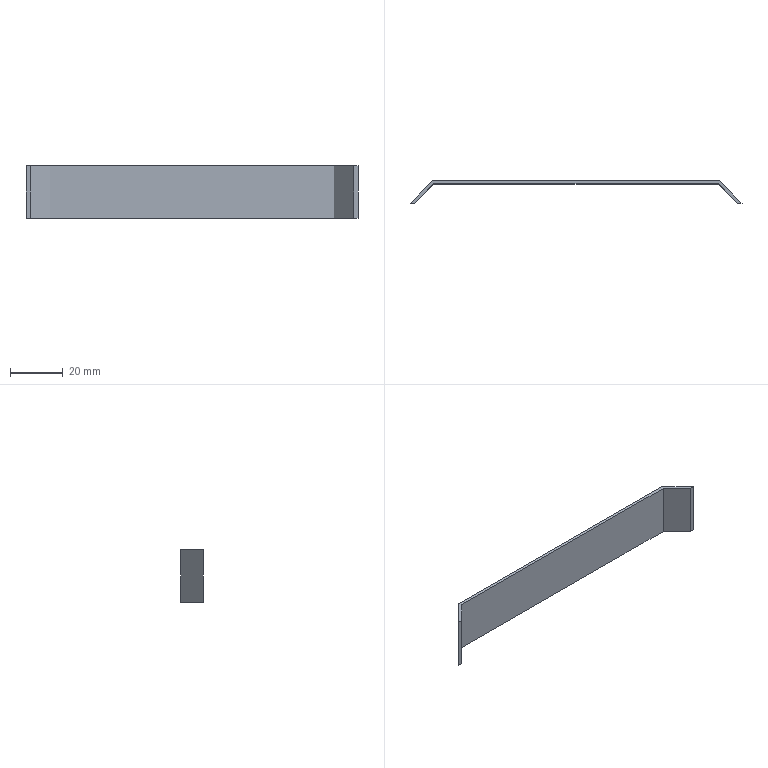Part | SolidWorks | features BaseBody 1 | 1 solid | 10 faces | box 126 x 8.5 x 20 mm | volume 3140 mm3 | plane 10
STEP:
#1=CARTESIAN_POINT('',(63.,-8.5,-10.));
#2=VERTEX_POINT('',#1);
#3=CARTESIAN_POINT('',(54.5,0.,-10.));
#4=VERTEX_POINT('',#3);
#5=CARTESIAN_POINT('',(54.5,0.,-10.));
#6=DIRECTION('',(-0.7071,0.7071,0.));
#7=VECTOR('',#6,1000.);
#8=LINE('',#5,#7);
#9=EDGE_CURVE('',#2,#4,#8,.T.);
#10=ORIENTED_EDGE('',*,*,#9,.F.);
#11=CARTESIAN_POINT('',(61.303,-8.5,-10.));
#12=VERTEX_POINT('',#11);
#13=CARTESIAN_POINT('',(63.,-8.5,-10.));
#14=DIRECTION('',(1.,0.,0.));
#15=VECTOR('',#14,1000.);
#16=LINE('',#13,#15);
#17=EDGE_CURVE('',#12,#2,#16,.T.);
#18=ORIENTED_EDGE('',*,*,#17,.F.);
#19=CARTESIAN_POINT('',(54.003,-1.2,-10.));
#20=VERTEX_POINT('',#19);
#21=CARTESIAN_POINT('',(54.003,-1.2,-10.));
#22=DIRECTION('',(0.7071,-0.7071,0.));
#23=VECTOR('',#22,1000.);
#24=LINE('',#21,#23);
#25=EDGE_CURVE('',#20,#12,#24,.T.);
#26=ORIENTED_EDGE('',*,*,#25,.F.);
#27=CARTESIAN_POINT('',(-54.003,-1.2,-10.));
#28=VERTEX_POINT('',#27);
#29=CARTESIAN_POINT('',(0.,-1.2,-10.));
#30=DIRECTION('',(1.,0.,0.));
#31=VECTOR('',#30,1000.);
#32=LINE('',#29,#31);
#33=EDGE_CURVE('',#28,#20,#32,.T.);
#34=ORIENTED_EDGE('',*,*,#33,.F.);
#35=CARTESIAN_POINT('',(-61.303,-8.5,-10.));
#36=VERTEX_POINT('',#35);
#37=CARTESIAN_POINT('',(-54.003,-1.2,-10.));
#38=DIRECTION('',(0.7071,0.7071,0.));
#39=VECTOR('',#38,1000.);
#40=LINE('',#37,#39);
#41=EDGE_CURVE('',#36,#28,#40,.T.);
#42=ORIENTED_EDGE('',*,*,#41,.F.);
#43=CARTESIAN_POINT('',(-63.,-8.5,-10.));
#44=VERTEX_POINT('',#43);
#45=CARTESIAN_POINT('',(-63.,-8.5,-10.));
#46=DIRECTION('',(1.,0.,0.));
#47=VECTOR('',#46,1000.);
#48=LINE('',#45,#47);
#49=EDGE_CURVE('',#44,#36,#48,.T.);
#50=ORIENTED_EDGE('',*,*,#49,.F.);
#51=CARTESIAN_POINT('',(-54.5,0.,-10.));
#52=VERTEX_POINT('',#51);
#53=CARTESIAN_POINT('',(-54.5,0.,-10.));
#54=DIRECTION('',(-0.7071,-0.7071,0.));
#55=VECTOR('',#54,1000.);
#56=LINE('',#53,#55);
#57=EDGE_CURVE('',#52,#44,#56,.T.);
#58=ORIENTED_EDGE('',*,*,#57,.F.);
#59=CARTESIAN_POINT('',(0.,0.,-10.));
#60=DIRECTION('',(-1.,0.,0.));
#61=VECTOR('',#60,1000.);
#62=LINE('',#59,#61);
#63=EDGE_CURVE('',#4,#52,#62,.T.);
#64=ORIENTED_EDGE('',*,*,#63,.F.);
#65=EDGE_LOOP('',(#10,#18,#26,#34,#42,#50,#58,#64));
#66=FACE_OUTER_BOUND('',#65,.T.);
#67=CARTESIAN_POINT('',(0.,0.,-10.));
#68=DIRECTION('',(0.,0.,-1.));
#69=DIRECTION('',(0.,-1.,0.));
#70=AXIS2_PLACEMENT_3D('',#67,#68,#69);
#71=PLANE('',#70);
#72=ADVANCED_FACE('',(#66),#71,.T.);
#73=CARTESIAN_POINT('',(63.,-8.5,10.));
#74=VERTEX_POINT('',#73);
#75=CARTESIAN_POINT('',(54.5,0.,10.));
#76=VERTEX_POINT('',#75);
#77=CARTESIAN_POINT('',(54.5,0.,10.));
#78=DIRECTION('',(-0.7071,0.7071,0.));
#79=VECTOR('',#78,1000.);
#80=LINE('',#77,#79);
#81=EDGE_CURVE('',#74,#76,#80,.T.);
#82=ORIENTED_EDGE('',*,*,#81,.T.);
#83=CARTESIAN_POINT('',(-54.5,0.,10.));
#84=VERTEX_POINT('',#83);
#85=CARTESIAN_POINT('',(0.,0.,10.));
#86=DIRECTION('',(-1.,0.,0.));
#87=VECTOR('',#86,1000.);
#88=LINE('',#85,#87);
#89=EDGE_CURVE('',#76,#84,#88,.T.);
#90=ORIENTED_EDGE('',*,*,#89,.T.);
#91=CARTESIAN_POINT('',(-63.,-8.5,10.));
#92=VERTEX_POINT('',#91);
#93=CARTESIAN_POINT('',(-54.5,0.,10.));
#94=DIRECTION('',(-0.7071,-0.7071,0.));
#95=VECTOR('',#94,1000.);
#96=LINE('',#93,#95);
#97=EDGE_CURVE('',#84,#92,#96,.T.);
#98=ORIENTED_EDGE('',*,*,#97,.T.);
#99=CARTESIAN_POINT('',(-61.303,-8.5,10.));
#100=VERTEX_POINT('',#99);
#101=CARTESIAN_POINT('',(-63.,-8.5,10.));
#102=DIRECTION('',(1.,0.,0.));
#103=VECTOR('',#102,1000.);
#104=LINE('',#101,#103);
#105=EDGE_CURVE('',#92,#100,#104,.T.);
#106=ORIENTED_EDGE('',*,*,#105,.T.);
#107=CARTESIAN_POINT('',(-54.003,-1.2,10.));
#108=VERTEX_POINT('',#107);
#109=CARTESIAN_POINT('',(-54.003,-1.2,10.));
#110=DIRECTION('',(0.7071,0.7071,0.));
#111=VECTOR('',#110,1000.);
#112=LINE('',#109,#111);
#113=EDGE_CURVE('',#100,#108,#112,.T.);
#114=ORIENTED_EDGE('',*,*,#113,.T.);
#115=CARTESIAN_POINT('',(54.003,-1.2,10.));
#116=VERTEX_POINT('',#115);
#117=CARTESIAN_POINT('',(0.,-1.2,10.));
#118=DIRECTION('',(1.,0.,0.));
#119=VECTOR('',#118,1000.);
#120=LINE('',#117,#119);
#121=EDGE_CURVE('',#108,#116,#120,.T.);
#122=ORIENTED_EDGE('',*,*,#121,.T.);
#123=CARTESIAN_POINT('',(61.303,-8.5,10.));
#124=VERTEX_POINT('',#123);
#125=CARTESIAN_POINT('',(54.003,-1.2,10.));
#126=DIRECTION('',(0.7071,-0.7071,0.));
#127=VECTOR('',#126,1000.);
#128=LINE('',#125,#127);
#129=EDGE_CURVE('',#116,#124,#128,.T.);
#130=ORIENTED_EDGE('',*,*,#129,.T.);
#131=CARTESIAN_POINT('',(63.,-8.5,10.));
#132=DIRECTION('',(1.,0.,0.));
#133=VECTOR('',#132,1000.);
#134=LINE('',#131,#133);
#135=EDGE_CURVE('',#124,#74,#134,.T.);
#136=ORIENTED_EDGE('',*,*,#135,.T.);
#137=EDGE_LOOP('',(#82,#90,#98,#106,#114,#122,#130,#136));
#138=FACE_OUTER_BOUND('',#137,.T.);
#139=CARTESIAN_POINT('',(0.,0.,10.));
#140=DIRECTION('',(0.,0.,-1.));
#141=DIRECTION('',(0.,-1.,0.));
#142=AXIS2_PLACEMENT_3D('',#139,#140,#141);
#143=PLANE('',#142);
#144=ADVANCED_FACE('',(#138),#143,.F.);
#145=ORIENTED_EDGE('',*,*,#17,.T.);
#146=CARTESIAN_POINT('',(63.,-8.5,10.));
#147=DIRECTION('',(0.,0.,-1.));
#148=VECTOR('',#147,1000.);
#149=LINE('',#146,#148);
#150=EDGE_CURVE('',#74,#2,#149,.T.);
#151=ORIENTED_EDGE('',*,*,#150,.F.);
#152=ORIENTED_EDGE('',*,*,#135,.F.);
#153=CARTESIAN_POINT('',(61.303,-8.5,10.));
#154=DIRECTION('',(0.,0.,-1.));
#155=VECTOR('',#154,1000.);
#156=LINE('',#153,#155);
#157=EDGE_CURVE('',#124,#12,#156,.T.);
#158=ORIENTED_EDGE('',*,*,#157,.T.);
#159=EDGE_LOOP('',(#145,#151,#152,#158));
#160=FACE_OUTER_BOUND('',#159,.T.);
#161=CARTESIAN_POINT('',(63.,-8.5,10.));
#162=DIRECTION('',(0.,1.,0.));
#163=DIRECTION('',(1.,0.,0.));
#164=AXIS2_PLACEMENT_3D('',#161,#162,#163);
#165=PLANE('',#164);
#166=ADVANCED_FACE('',(#160),#165,.F.);
#167=ORIENTED_EDGE('',*,*,#25,.T.);
#168=ORIENTED_EDGE('',*,*,#157,.F.);
#169=ORIENTED_EDGE('',*,*,#129,.F.);
#170=CARTESIAN_POINT('',(54.003,-1.2,10.));
#171=DIRECTION('',(0.,0.,-1.));
#172=VECTOR('',#171,1000.);
#173=LINE('',#170,#172);
#174=EDGE_CURVE('',#116,#20,#173,.T.);
#175=ORIENTED_EDGE('',*,*,#174,.T.);
#176=EDGE_LOOP('',(#167,#168,#169,#175));
#177=FACE_OUTER_BOUND('',#176,.T.);
#178=CARTESIAN_POINT('',(54.003,-1.2,10.));
#179=DIRECTION('',(0.7071,0.7071,0.));
#180=DIRECTION('',(0.,0.,-1.));
#181=AXIS2_PLACEMENT_3D('',#178,#179,#180);
#182=PLANE('',#181);
#183=ADVANCED_FACE('',(#177),#182,.F.);
#184=ORIENTED_EDGE('',*,*,#33,.T.);
#185=ORIENTED_EDGE('',*,*,#174,.F.);
#186=ORIENTED_EDGE('',*,*,#121,.F.);
#187=CARTESIAN_POINT('',(-54.003,-1.2,10.));
#188=DIRECTION('',(0.,0.,-1.));
#189=VECTOR('',#188,1000.);
#190=LINE('',#187,#189);
#191=EDGE_CURVE('',#108,#28,#190,.T.);
#192=ORIENTED_EDGE('',*,*,#191,.T.);
#193=EDGE_LOOP('',(#184,#185,#186,#192));
#194=FACE_OUTER_BOUND('',#193,.T.);
#195=CARTESIAN_POINT('',(0.,-1.2,10.));
#196=DIRECTION('',(0.,1.,0.));
#197=DIRECTION('',(1.,0.,0.));
#198=AXIS2_PLACEMENT_3D('',#195,#196,#197);
#199=PLANE('',#198);
#200=ADVANCED_FACE('',(#194),#199,.F.);
#201=ORIENTED_EDGE('',*,*,#41,.T.);
#202=ORIENTED_EDGE('',*,*,#191,.F.);
#203=ORIENTED_EDGE('',*,*,#113,.F.);
#204=CARTESIAN_POINT('',(-61.303,-8.5,10.));
#205=DIRECTION('',(0.,0.,-1.));
#206=VECTOR('',#205,1000.);
#207=LINE('',#204,#206);
#208=EDGE_CURVE('',#100,#36,#207,.T.);
#209=ORIENTED_EDGE('',*,*,#208,.T.);
#210=EDGE_LOOP('',(#201,#202,#203,#209));
#211=FACE_OUTER_BOUND('',#210,.T.);
#212=CARTESIAN_POINT('',(-54.003,-1.2,10.));
#213=DIRECTION('',(-0.7071,0.7071,0.));
#214=DIRECTION('',(0.,0.,1.));
#215=AXIS2_PLACEMENT_3D('',#212,#213,#214);
#216=PLANE('',#215);
#217=ADVANCED_FACE('',(#211),#216,.F.);
#218=ORIENTED_EDGE('',*,*,#49,.T.);
#219=ORIENTED_EDGE('',*,*,#208,.F.);
#220=ORIENTED_EDGE('',*,*,#105,.F.);
#221=CARTESIAN_POINT('',(-63.,-8.5,10.));
#222=DIRECTION('',(0.,0.,-1.));
#223=VECTOR('',#222,1000.);
#224=LINE('',#221,#223);
#225=EDGE_CURVE('',#92,#44,#224,.T.);
#226=ORIENTED_EDGE('',*,*,#225,.T.);
#227=EDGE_LOOP('',(#218,#219,#220,#226));
#228=FACE_OUTER_BOUND('',#227,.T.);
#229=CARTESIAN_POINT('',(-63.,-8.5,10.));
#230=DIRECTION('',(0.,1.,0.));
#231=DIRECTION('',(1.,0.,0.));
#232=AXIS2_PLACEMENT_3D('',#229,#230,#231);
#233=PLANE('',#232);
#234=ADVANCED_FACE('',(#228),#233,.F.);
#235=ORIENTED_EDGE('',*,*,#57,.T.);
#236=ORIENTED_EDGE('',*,*,#225,.F.);
#237=ORIENTED_EDGE('',*,*,#97,.F.);
#238=CARTESIAN_POINT('',(-54.5,0.,10.));
#239=DIRECTION('',(0.,0.,-1.));
#240=VECTOR('',#239,1000.);
#241=LINE('',#238,#240);
#242=EDGE_CURVE('',#84,#52,#241,.T.);
#243=ORIENTED_EDGE('',*,*,#242,.T.);
#244=EDGE_LOOP('',(#235,#236,#237,#243));
#245=FACE_OUTER_BOUND('',#244,.T.);
#246=CARTESIAN_POINT('',(-54.5,0.,10.));
#247=DIRECTION('',(0.7071,-0.7071,0.));
#248=DIRECTION('',(0.,0.,-1.));
#249=AXIS2_PLACEMENT_3D('',#246,#247,#248);
#250=PLANE('',#249);
#251=ADVANCED_FACE('',(#245),#250,.F.);
#252=ORIENTED_EDGE('',*,*,#63,.T.);
#253=ORIENTED_EDGE('',*,*,#242,.F.);
#254=ORIENTED_EDGE('',*,*,#89,.F.);
#255=CARTESIAN_POINT('',(54.5,0.,10.));
#256=DIRECTION('',(0.,0.,-1.));
#257=VECTOR('',#256,1000.);
#258=LINE('',#255,#257);
#259=EDGE_CURVE('',#76,#4,#258,.T.);
#260=ORIENTED_EDGE('',*,*,#259,.T.);
#261=EDGE_LOOP('',(#252,#253,#254,#260));
#262=FACE_OUTER_BOUND('',#261,.T.);
#263=CARTESIAN_POINT('',(0.,0.,10.));
#264=DIRECTION('',(0.,-1.,0.));
#265=DIRECTION('',(0.,0.,-1.));
#266=AXIS2_PLACEMENT_3D('',#263,#264,#265);
#267=PLANE('',#266);
#268=ADVANCED_FACE('',(#262),#267,.F.);
#269=ORIENTED_EDGE('',*,*,#9,.T.);
#270=ORIENTED_EDGE('',*,*,#259,.F.);
#271=ORIENTED_EDGE('',*,*,#81,.F.);
#272=ORIENTED_EDGE('',*,*,#150,.T.);
#273=EDGE_LOOP('',(#269,#270,#271,#272));
#274=FACE_OUTER_BOUND('',#273,.T.);
#275=CARTESIAN_POINT('',(54.5,0.,10.));
#276=DIRECTION('',(-0.7071,-0.7071,0.));
#277=DIRECTION('',(-0.7071,0.7071,0.));
#278=AXIS2_PLACEMENT_3D('',#275,#276,#277);
#279=PLANE('',#278);
#280=ADVANCED_FACE('',(#274),#279,.F.);
#281=CLOSED_SHELL('',(#72,#144,#166,#183,#200,#217,#234,#251,#268,#280));
#282=MANIFOLD_SOLID_BREP('',#281);
#283=CARTESIAN_POINT('',(0.,0.,0.));
#284=DIRECTION('',(0.,0.,1.));
#285=DIRECTION('',(1.,0.,0.));
#286=AXIS2_PLACEMENT_3D('',#283,#284,#285);
#287=(LENGTH_UNIT()NAMED_UNIT(*)SI_UNIT(.MILLI.,.METRE.));
#288=UNCERTAINTY_MEASURE_WITH_UNIT(LENGTH_MEASURE(0.00001),#287,'','');
#289=(NAMED_UNIT(*)PLANE_ANGLE_UNIT()SI_UNIT($,.RADIAN.));
#290=(NAMED_UNIT(*)SI_UNIT($,.STERADIAN.)SOLID_ANGLE_UNIT());
#291=(GEOMETRIC_REPRESENTATION_CONTEXT(3)GLOBAL_UNCERTAINTY_ASSIGNED_CONTEXT((#288))GLOBAL_UNIT_ASSIGNED_CONTEXT((#287,#289,#290))REPRESENTATION_CONTEXT('',''));
#292=ADVANCED_BREP_SHAPE_REPRESENTATION('',(#282,#286),#291);